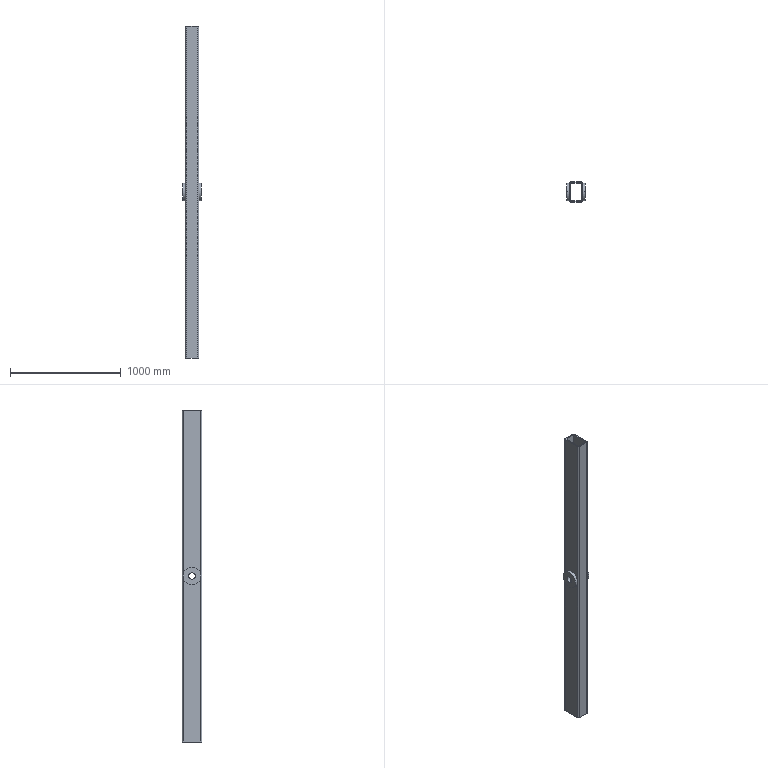Part | SolidWorks | features ICE 2, Extrusion 1, MirrorPattern 1 | 1 solid | 34 faces | box 170 x 180 x 3000 mm | volume 17246858 mm3 | plane 18 | cylinder 16 | commonest cylinder face diameters 4 x4 24 x4 60 x4 160 x4
STEP:
#1=CARTESIAN_POINT('',(-85.,0.,-80.));
#2=VERTEX_POINT('',#1);
#3=CARTESIAN_POINT('',(-85.,0.,80.));
#4=VERTEX_POINT('',#3);
#5=CARTESIAN_POINT('',(-85.,0.,0.));
#6=DIRECTION('',(1.,0.,0.));
#7=DIRECTION('',(0.,0.,-1.));
#8=AXIS2_PLACEMENT_3D('',#5,#6,#7);
#9=CIRCLE('',#8,80.);
#10=EDGE_CURVE('',#2,#4,#9,.T.);
#11=ORIENTED_EDGE('',*,*,#10,.T.);
#12=CARTESIAN_POINT('',(-60.,0.,80.));
#13=VERTEX_POINT('',#12);
#14=CARTESIAN_POINT('',(-85.,0.,80.));
#15=DIRECTION('',(1.,0.,0.));
#16=VECTOR('',#15,1000.);
#17=LINE('',#14,#16);
#18=EDGE_CURVE('',#4,#13,#17,.T.);
#19=ORIENTED_EDGE('',*,*,#18,.T.);
#20=CARTESIAN_POINT('',(-60.,78.,17.776));
#21=VERTEX_POINT('',#20);
#22=CARTESIAN_POINT('',(-60.,0.,0.));
#23=DIRECTION('',(1.,0.,0.));
#24=DIRECTION('',(0.,0.,-1.));
#25=AXIS2_PLACEMENT_3D('',#22,#23,#24);
#26=CIRCLE('',#25,80.);
#27=EDGE_CURVE('',#21,#13,#26,.T.);
#28=ORIENTED_EDGE('',*,*,#27,.F.);
#29=CARTESIAN_POINT('',(-60.,78.,-17.776));
#30=VERTEX_POINT('',#29);
#31=CARTESIAN_POINT('',(-60.,0.,0.));
#32=DIRECTION('',(1.,0.,0.));
#33=DIRECTION('',(0.,0.,-1.));
#34=AXIS2_PLACEMENT_3D('',#31,#32,#33);
#35=CIRCLE('',#34,80.);
#36=EDGE_CURVE('',#30,#21,#35,.T.);
#37=ORIENTED_EDGE('',*,*,#36,.F.);
#38=CARTESIAN_POINT('',(-60.,0.,-80.));
#39=VERTEX_POINT('',#38);
#40=CARTESIAN_POINT('',(-60.,0.,0.));
#41=DIRECTION('',(1.,0.,0.));
#42=DIRECTION('',(0.,0.,-1.));
#43=AXIS2_PLACEMENT_3D('',#40,#41,#42);
#44=CIRCLE('',#43,80.);
#45=EDGE_CURVE('',#39,#30,#44,.T.);
#46=ORIENTED_EDGE('',*,*,#45,.F.);
#47=CARTESIAN_POINT('',(-85.,0.,-80.));
#48=DIRECTION('',(1.,0.,0.));
#49=VECTOR('',#48,1000.);
#50=LINE('',#47,#49);
#51=EDGE_CURVE('',#2,#39,#50,.T.);
#52=ORIENTED_EDGE('',*,*,#51,.F.);
#53=EDGE_LOOP('',(#11,#19,#28,#37,#46,#52));
#54=FACE_OUTER_BOUND('',#53,.T.);
#55=CARTESIAN_POINT('',(-85.,0.,0.));
#56=DIRECTION('',(1.,0.,0.));
#57=DIRECTION('',(0.,0.,-1.));
#58=AXIS2_PLACEMENT_3D('',#55,#56,#57);
#59=CYLINDRICAL_SURFACE('',#58,80.);
#60=ADVANCED_FACE('',(#54),#59,.T.);
#61=CARTESIAN_POINT('',(85.,0.,-80.));
#62=VERTEX_POINT('',#61);
#63=CARTESIAN_POINT('',(85.,0.,80.));
#64=VERTEX_POINT('',#63);
#65=CARTESIAN_POINT('',(85.,0.,0.));
#66=DIRECTION('',(1.,0.,0.));
#67=DIRECTION('',(0.,0.,-1.));
#68=AXIS2_PLACEMENT_3D('',#65,#66,#67);
#69=CIRCLE('',#68,80.);
#70=EDGE_CURVE('',#62,#64,#69,.T.);
#71=ORIENTED_EDGE('',*,*,#70,.F.);
#72=CARTESIAN_POINT('',(60.,0.,-80.));
#73=VERTEX_POINT('',#72);
#74=CARTESIAN_POINT('',(85.,0.,-80.));
#75=DIRECTION('',(-1.,0.,0.));
#76=VECTOR('',#75,1000.);
#77=LINE('',#74,#76);
#78=EDGE_CURVE('',#62,#73,#77,.T.);
#79=ORIENTED_EDGE('',*,*,#78,.T.);
#80=CARTESIAN_POINT('',(60.,78.,-17.776));
#81=VERTEX_POINT('',#80);
#82=CARTESIAN_POINT('',(60.,0.,0.));
#83=DIRECTION('',(1.,0.,0.));
#84=DIRECTION('',(0.,0.,-1.));
#85=AXIS2_PLACEMENT_3D('',#82,#83,#84);
#86=CIRCLE('',#85,80.);
#87=EDGE_CURVE('',#73,#81,#86,.T.);
#88=ORIENTED_EDGE('',*,*,#87,.T.);
#89=CARTESIAN_POINT('',(60.,78.,17.776));
#90=VERTEX_POINT('',#89);
#91=CARTESIAN_POINT('',(60.,0.,0.));
#92=DIRECTION('',(1.,0.,0.));
#93=DIRECTION('',(0.,0.,-1.));
#94=AXIS2_PLACEMENT_3D('',#91,#92,#93);
#95=CIRCLE('',#94,80.);
#96=EDGE_CURVE('',#81,#90,#95,.T.);
#97=ORIENTED_EDGE('',*,*,#96,.T.);
#98=CARTESIAN_POINT('',(60.,0.,80.));
#99=VERTEX_POINT('',#98);
#100=CARTESIAN_POINT('',(60.,0.,0.));
#101=DIRECTION('',(1.,0.,0.));
#102=DIRECTION('',(0.,0.,-1.));
#103=AXIS2_PLACEMENT_3D('',#100,#101,#102);
#104=CIRCLE('',#103,80.);
#105=EDGE_CURVE('',#90,#99,#104,.T.);
#106=ORIENTED_EDGE('',*,*,#105,.T.);
#107=CARTESIAN_POINT('',(85.,0.,80.));
#108=DIRECTION('',(-1.,0.,0.));
#109=VECTOR('',#108,1000.);
#110=LINE('',#107,#109);
#111=EDGE_CURVE('',#64,#99,#110,.T.);
#112=ORIENTED_EDGE('',*,*,#111,.F.);
#113=EDGE_LOOP('',(#71,#79,#88,#97,#106,#112));
#114=FACE_OUTER_BOUND('',#113,.T.);
#115=CARTESIAN_POINT('',(85.,0.,0.));
#116=DIRECTION('',(-1.,0.,0.));
#117=DIRECTION('',(0.,0.,1.));
#118=AXIS2_PLACEMENT_3D('',#115,#116,#117);
#119=CYLINDRICAL_SURFACE('',#118,80.);
#120=ADVANCED_FACE('',(#114),#119,.T.);
#121=CARTESIAN_POINT('',(-85.,0.,30.));
#122=VERTEX_POINT('',#121);
#123=CARTESIAN_POINT('',(-85.,0.,-30.));
#124=VERTEX_POINT('',#123);
#125=CARTESIAN_POINT('',(-85.,0.,0.));
#126=DIRECTION('',(1.,0.,0.));
#127=DIRECTION('',(0.,0.,-1.));
#128=AXIS2_PLACEMENT_3D('',#125,#126,#127);
#129=CIRCLE('',#128,30.);
#130=EDGE_CURVE('',#122,#124,#129,.T.);
#131=ORIENTED_EDGE('',*,*,#130,.F.);
#132=CARTESIAN_POINT('',(-50.,0.,30.));
#133=VERTEX_POINT('',#132);
#134=CARTESIAN_POINT('',(-60.,0.,30.));
#135=DIRECTION('',(1.,0.,0.));
#136=VECTOR('',#135,1000.);
#137=LINE('',#134,#136);
#138=EDGE_CURVE('',#122,#133,#137,.T.);
#139=ORIENTED_EDGE('',*,*,#138,.T.);
#140=CARTESIAN_POINT('',(-50.,0.,-30.));
#141=VERTEX_POINT('',#140);
#142=CARTESIAN_POINT('',(-50.,0.,0.));
#143=DIRECTION('',(1.,0.,0.));
#144=DIRECTION('',(0.,1.,0.));
#145=AXIS2_PLACEMENT_3D('',#142,#143,#144);
#146=CIRCLE('',#145,30.);
#147=EDGE_CURVE('',#133,#141,#146,.T.);
#148=ORIENTED_EDGE('',*,*,#147,.T.);
#149=CARTESIAN_POINT('',(-60.,0.,-30.));
#150=DIRECTION('',(1.,0.,0.));
#151=VECTOR('',#150,1000.);
#152=LINE('',#149,#151);
#153=EDGE_CURVE('',#124,#141,#152,.T.);
#154=ORIENTED_EDGE('',*,*,#153,.F.);
#155=EDGE_LOOP('',(#131,#139,#148,#154));
#156=FACE_OUTER_BOUND('',#155,.T.);
#157=CARTESIAN_POINT('',(-60.,0.,0.));
#158=DIRECTION('',(1.,0.,0.));
#159=DIRECTION('',(0.,0.,-1.));
#160=AXIS2_PLACEMENT_3D('',#157,#158,#159);
#161=CYLINDRICAL_SURFACE('',#160,30.);
#162=ADVANCED_FACE('',(#156),#161,.F.);
#163=CARTESIAN_POINT('',(50.,0.,-30.));
#164=VERTEX_POINT('',#163);
#165=CARTESIAN_POINT('',(50.,0.,30.));
#166=VERTEX_POINT('',#165);
#167=CARTESIAN_POINT('',(50.,0.,0.));
#168=DIRECTION('',(-1.,0.,0.));
#169=DIRECTION('',(0.,0.,1.));
#170=AXIS2_PLACEMENT_3D('',#167,#168,#169);
#171=CIRCLE('',#170,30.);
#172=EDGE_CURVE('',#164,#166,#171,.T.);
#173=ORIENTED_EDGE('',*,*,#172,.T.);
#174=CARTESIAN_POINT('',(85.,0.,30.));
#175=VERTEX_POINT('',#174);
#176=CARTESIAN_POINT('',(-60.,0.,30.));
#177=DIRECTION('',(1.,0.,0.));
#178=VECTOR('',#177,1000.);
#179=LINE('',#176,#178);
#180=EDGE_CURVE('',#166,#175,#179,.T.);
#181=ORIENTED_EDGE('',*,*,#180,.T.);
#182=CARTESIAN_POINT('',(85.,0.,-30.));
#183=VERTEX_POINT('',#182);
#184=CARTESIAN_POINT('',(85.,0.,0.));
#185=DIRECTION('',(1.,0.,0.));
#186=DIRECTION('',(0.,0.,-1.));
#187=AXIS2_PLACEMENT_3D('',#184,#185,#186);
#188=CIRCLE('',#187,30.);
#189=EDGE_CURVE('',#175,#183,#188,.T.);
#190=ORIENTED_EDGE('',*,*,#189,.T.);
#191=CARTESIAN_POINT('',(-60.,0.,-30.));
#192=DIRECTION('',(1.,0.,0.));
#193=VECTOR('',#192,1000.);
#194=LINE('',#191,#193);
#195=EDGE_CURVE('',#164,#183,#194,.T.);
#196=ORIENTED_EDGE('',*,*,#195,.F.);
#197=EDGE_LOOP('',(#173,#181,#190,#196));
#198=FACE_OUTER_BOUND('',#197,.T.);
#199=CARTESIAN_POINT('',(-60.,0.,0.));
#200=DIRECTION('',(1.,0.,0.));
#201=DIRECTION('',(0.,0.,-1.));
#202=AXIS2_PLACEMENT_3D('',#199,#200,#201);
#203=CYLINDRICAL_SURFACE('',#202,30.);
#204=ADVANCED_FACE('',(#198),#203,.F.);
#205=CARTESIAN_POINT('',(-60.,78.,1500.));
#206=VERTEX_POINT('',#205);
#207=CARTESIAN_POINT('',(-60.,78.,1500.));
#208=DIRECTION('',(0.,0.,-1.));
#209=VECTOR('',#208,1000.);
#210=LINE('',#207,#209);
#211=EDGE_CURVE('',#206,#21,#210,.T.);
#212=ORIENTED_EDGE('',*,*,#211,.T.);
#213=ORIENTED_EDGE('',*,*,#27,.T.);
#214=CARTESIAN_POINT('',(-60.,-78.,17.776));
#215=VERTEX_POINT('',#214);
#216=CARTESIAN_POINT('',(-60.,0.,0.));
#217=DIRECTION('',(1.,0.,0.));
#218=DIRECTION('',(0.,0.,-1.));
#219=AXIS2_PLACEMENT_3D('',#216,#217,#218);
#220=CIRCLE('',#219,80.);
#221=EDGE_CURVE('',#13,#215,#220,.T.);
#222=ORIENTED_EDGE('',*,*,#221,.T.);
#223=CARTESIAN_POINT('',(-60.,-78.,1500.));
#224=VERTEX_POINT('',#223);
#225=CARTESIAN_POINT('',(-60.,-78.,1500.));
#226=DIRECTION('',(0.,0.,-1.));
#227=VECTOR('',#226,1000.);
#228=LINE('',#225,#227);
#229=EDGE_CURVE('',#224,#215,#228,.T.);
#230=ORIENTED_EDGE('',*,*,#229,.F.);
#231=CARTESIAN_POINT('',(-60.,78.,1500.));
#232=DIRECTION('',(0.,-1.,0.));
#233=VECTOR('',#232,1000.);
#234=LINE('',#231,#233);
#235=EDGE_CURVE('',#206,#224,#234,.T.);
#236=ORIENTED_EDGE('',*,*,#235,.F.);
#237=EDGE_LOOP('',(#212,#213,#222,#230,#236));
#238=FACE_OUTER_BOUND('',#237,.T.);
#239=CARTESIAN_POINT('',(-60.,-78.,1500.));
#240=DIRECTION('',(1.,0.,0.));
#241=DIRECTION('',(0.,1.,0.));
#242=AXIS2_PLACEMENT_3D('',#239,#240,#241);
#243=PLANE('',#242);
#244=ADVANCED_FACE('',(#238),#243,.F.);
#245=CARTESIAN_POINT('',(60.,-78.,-17.776));
#246=VERTEX_POINT('',#245);
#247=CARTESIAN_POINT('',(60.,0.,0.));
#248=DIRECTION('',(1.,0.,0.));
#249=DIRECTION('',(0.,0.,-1.));
#250=AXIS2_PLACEMENT_3D('',#247,#248,#249);
#251=CIRCLE('',#250,80.);
#252=EDGE_CURVE('',#246,#73,#251,.T.);
#253=ORIENTED_EDGE('',*,*,#252,.F.);
#254=CARTESIAN_POINT('',(60.,-78.,-1500.));
#255=VERTEX_POINT('',#254);
#256=CARTESIAN_POINT('',(60.,-78.,1500.));
#257=DIRECTION('',(0.,0.,-1.));
#258=VECTOR('',#257,1000.);
#259=LINE('',#256,#258);
#260=EDGE_CURVE('',#246,#255,#259,.T.);
#261=ORIENTED_EDGE('',*,*,#260,.T.);
#262=CARTESIAN_POINT('',(60.,78.,-1500.));
#263=VERTEX_POINT('',#262);
#264=CARTESIAN_POINT('',(60.,78.,-1500.));
#265=DIRECTION('',(0.,1.,0.));
#266=VECTOR('',#265,1000.);
#267=LINE('',#264,#266);
#268=EDGE_CURVE('',#255,#263,#267,.T.);
#269=ORIENTED_EDGE('',*,*,#268,.T.);
#270=CARTESIAN_POINT('',(60.,78.,1500.));
#271=DIRECTION('',(0.,0.,-1.));
#272=VECTOR('',#271,1000.);
#273=LINE('',#270,#272);
#274=EDGE_CURVE('',#81,#263,#273,.T.);
#275=ORIENTED_EDGE('',*,*,#274,.F.);
#276=ORIENTED_EDGE('',*,*,#87,.F.);
#277=EDGE_LOOP('',(#253,#261,#269,#275,#276));
#278=FACE_OUTER_BOUND('',#277,.T.);
#279=CARTESIAN_POINT('',(60.,78.,1500.));
#280=DIRECTION('',(-1.,0.,0.));
#281=DIRECTION('',(0.,0.,1.));
#282=AXIS2_PLACEMENT_3D('',#279,#280,#281);
#283=PLANE('',#282);
#284=ADVANCED_FACE('',(#278),#283,.F.);
#285=ORIENTED_EDGE('',*,*,#105,.F.);
#286=CARTESIAN_POINT('',(60.,78.,1500.));
#287=VERTEX_POINT('',#286);
#288=CARTESIAN_POINT('',(60.,78.,1500.));
#289=DIRECTION('',(0.,0.,-1.));
#290=VECTOR('',#289,1000.);
#291=LINE('',#288,#290);
#292=EDGE_CURVE('',#287,#90,#291,.T.);
#293=ORIENTED_EDGE('',*,*,#292,.F.);
#294=CARTESIAN_POINT('',(60.,-78.,1500.));
#295=VERTEX_POINT('',#294);
#296=CARTESIAN_POINT('',(60.,78.,1500.));
#297=DIRECTION('',(0.,1.,0.));
#298=VECTOR('',#297,1000.);
#299=LINE('',#296,#298);
#300=EDGE_CURVE('',#295,#287,#299,.T.);
#301=ORIENTED_EDGE('',*,*,#300,.F.);
#302=CARTESIAN_POINT('',(60.,-78.,17.776));
#303=VERTEX_POINT('',#302);
#304=CARTESIAN_POINT('',(60.,-78.,1500.));
#305=DIRECTION('',(0.,0.,-1.));
#306=VECTOR('',#305,1000.);
#307=LINE('',#304,#306);
#308=EDGE_CURVE('',#295,#303,#307,.T.);
#309=ORIENTED_EDGE('',*,*,#308,.T.);
#310=CARTESIAN_POINT('',(60.,0.,0.));
#311=DIRECTION('',(1.,0.,0.));
#312=DIRECTION('',(0.,0.,-1.));
#313=AXIS2_PLACEMENT_3D('',#310,#311,#312);
#314=CIRCLE('',#313,80.);
#315=EDGE_CURVE('',#99,#303,#314,.T.);
#316=ORIENTED_EDGE('',*,*,#315,.F.);
#317=EDGE_LOOP('',(#285,#293,#301,#309,#316));
#318=FACE_OUTER_BOUND('',#317,.T.);
#319=CARTESIAN_POINT('',(60.,78.,1500.));
#320=DIRECTION('',(-1.,0.,0.));
#321=DIRECTION('',(0.,0.,1.));
#322=AXIS2_PLACEMENT_3D('',#319,#320,#321);
#323=PLANE('',#322);
#324=ADVANCED_FACE('',(#318),#323,.F.);
#325=CARTESIAN_POINT('',(-48.,90.,1500.));
#326=VERTEX_POINT('',#325);
#327=CARTESIAN_POINT('',(-48.,78.,1500.));
#328=DIRECTION('',(0.,0.,1.));
#329=DIRECTION('',(1.,0.,0.));
#330=AXIS2_PLACEMENT_3D('',#327,#328,#329);
#331=CIRCLE('',#330,12.);
#332=EDGE_CURVE('',#326,#206,#331,.T.);
#333=ORIENTED_EDGE('',*,*,#332,.T.);
#334=ORIENTED_EDGE('',*,*,#235,.T.);
#335=CARTESIAN_POINT('',(-48.,-90.,1500.));
#336=VERTEX_POINT('',#335);
#337=CARTESIAN_POINT('',(-48.,-78.,1500.));
#338=DIRECTION('',(0.,0.,1.));
#339=DIRECTION('',(-1.,0.,0.));
#340=AXIS2_PLACEMENT_3D('',#337,#338,#339);
#341=CIRCLE('',#340,12.);
#342=EDGE_CURVE('',#224,#336,#341,.T.);
#343=ORIENTED_EDGE('',*,*,#342,.T.);
#344=CARTESIAN_POINT('',(48.,-90.,1500.));
#345=VERTEX_POINT('',#344);
#346=CARTESIAN_POINT('',(0.,-90.,1500.));
#347=DIRECTION('',(1.,0.,0.));
#348=VECTOR('',#347,1000.);
#349=LINE('',#346,#348);
#350=EDGE_CURVE('',#336,#345,#349,.T.);
#351=ORIENTED_EDGE('',*,*,#350,.T.);
#352=CARTESIAN_POINT('',(48.,-78.,1500.));
#353=DIRECTION('',(0.,0.,1.));
#354=DIRECTION('',(1.,0.,0.));
#355=AXIS2_PLACEMENT_3D('',#352,#353,#354);
#356=CIRCLE('',#355,12.);
#357=EDGE_CURVE('',#345,#295,#356,.T.);
#358=ORIENTED_EDGE('',*,*,#357,.T.);
#359=ORIENTED_EDGE('',*,*,#300,.T.);
#360=CARTESIAN_POINT('',(48.,90.,1500.));
#361=VERTEX_POINT('',#360);
#362=CARTESIAN_POINT('',(48.,78.,1500.));
#363=DIRECTION('',(0.,0.,1.));
#364=DIRECTION('',(-1.,0.,0.));
#365=AXIS2_PLACEMENT_3D('',#362,#363,#364);
#366=CIRCLE('',#365,12.);
#367=EDGE_CURVE('',#287,#361,#366,.T.);
#368=ORIENTED_EDGE('',*,*,#367,.T.);
#369=CARTESIAN_POINT('',(0.,90.,1500.));
#370=DIRECTION('',(-1.,0.,0.));
#371=VECTOR('',#370,1000.);
#372=LINE('',#369,#371);
#373=EDGE_CURVE('',#361,#326,#372,.T.);
#374=ORIENTED_EDGE('',*,*,#373,.T.);
#375=EDGE_LOOP('',(#333,#334,#343,#351,#358,#359,#368,#374));
#376=FACE_OUTER_BOUND('',#375,.T.);
#377=CARTESIAN_POINT('',(-50.,78.,1500.));
#378=VERTEX_POINT('',#377);
#379=CARTESIAN_POINT('',(-50.,-78.,1500.));
#380=VERTEX_POINT('',#379);
#381=CARTESIAN_POINT('',(-50.,78.,1500.));
#382=DIRECTION('',(0.,-1.,0.));
#383=VECTOR('',#382,1000.);
#384=LINE('',#381,#383);
#385=EDGE_CURVE('',#378,#380,#384,.T.);
#386=ORIENTED_EDGE('',*,*,#385,.F.);
#387=CARTESIAN_POINT('',(-48.,80.,1500.));
#388=VERTEX_POINT('',#387);
#389=CARTESIAN_POINT('',(-48.,78.,1500.));
#390=DIRECTION('',(0.,0.,1.));
#391=DIRECTION('',(1.,0.,0.));
#392=AXIS2_PLACEMENT_3D('',#389,#390,#391);
#393=CIRCLE('',#392,2.);
#394=EDGE_CURVE('',#388,#378,#393,.T.);
#395=ORIENTED_EDGE('',*,*,#394,.F.);
#396=CARTESIAN_POINT('',(48.,80.,1500.));
#397=VERTEX_POINT('',#396);
#398=CARTESIAN_POINT('',(0.,80.,1500.));
#399=DIRECTION('',(-1.,0.,0.));
#400=VECTOR('',#399,1000.);
#401=LINE('',#398,#400);
#402=EDGE_CURVE('',#397,#388,#401,.T.);
#403=ORIENTED_EDGE('',*,*,#402,.F.);
#404=CARTESIAN_POINT('',(50.,78.,1500.));
#405=VERTEX_POINT('',#404);
#406=CARTESIAN_POINT('',(48.,78.,1500.));
#407=DIRECTION('',(0.,0.,1.));
#408=DIRECTION('',(-1.,0.,0.));
#409=AXIS2_PLACEMENT_3D('',#406,#407,#408);
#410=CIRCLE('',#409,2.);
#411=EDGE_CURVE('',#405,#397,#410,.T.);
#412=ORIENTED_EDGE('',*,*,#411,.F.);
#413=CARTESIAN_POINT('',(50.,-78.,1500.));
#414=VERTEX_POINT('',#413);
#415=CARTESIAN_POINT('',(50.,78.,1500.));
#416=DIRECTION('',(0.,1.,0.));
#417=VECTOR('',#416,1000.);
#418=LINE('',#415,#417);
#419=EDGE_CURVE('',#414,#405,#418,.T.);
#420=ORIENTED_EDGE('',*,*,#419,.F.);
#421=CARTESIAN_POINT('',(48.,-80.,1500.));
#422=VERTEX_POINT('',#421);
#423=CARTESIAN_POINT('',(48.,-78.,1500.));
#424=DIRECTION('',(0.,0.,1.));
#425=DIRECTION('',(1.,0.,0.));
#426=AXIS2_PLACEMENT_3D('',#423,#424,#425);
#427=CIRCLE('',#426,2.);
#428=EDGE_CURVE('',#422,#414,#427,.T.);
#429=ORIENTED_EDGE('',*,*,#428,.F.);
#430=CARTESIAN_POINT('',(-48.,-80.,1500.));
#431=VERTEX_POINT('',#430);
#432=CARTESIAN_POINT('',(0.,-80.,1500.));
#433=DIRECTION('',(1.,0.,0.));
#434=VECTOR('',#433,1000.);
#435=LINE('',#432,#434);
#436=EDGE_CURVE('',#431,#422,#435,.T.);
#437=ORIENTED_EDGE('',*,*,#436,.F.);
#438=CARTESIAN_POINT('',(-48.,-78.,1500.));
#439=DIRECTION('',(0.,0.,1.));
#440=DIRECTION('',(-1.,0.,0.));
#441=AXIS2_PLACEMENT_3D('',#438,#439,#440);
#442=CIRCLE('',#441,2.);
#443=EDGE_CURVE('',#380,#431,#442,.T.);
#444=ORIENTED_EDGE('',*,*,#443,.F.);
#445=EDGE_LOOP('',(#386,#395,#403,#412,#420,#429,#437,#444));
#446=FACE_BOUND('',#445,.T.);
#447=CARTESIAN_POINT('',(-48.,78.,1500.));
#448=DIRECTION('',(0.,0.,1.));
#449=DIRECTION('',(1.,0.,0.));
#450=AXIS2_PLACEMENT_3D('',#447,#448,#449);
#451=PLANE('',#450);
#452=ADVANCED_FACE('',(#376,#446),#451,.T.);
#453=CARTESIAN_POINT('',(-48.,90.,-1500.));
#454=VERTEX_POINT('',#453);
#455=CARTESIAN_POINT('',(-60.,78.,-1500.));
#456=VERTEX_POINT('',#455);
#457=CARTESIAN_POINT('',(-48.,78.,-1500.));
#458=DIRECTION('',(0.,0.,1.));
#459=DIRECTION('',(1.,0.,0.));
#460=AXIS2_PLACEMENT_3D('',#457,#458,#459);
#461=CIRCLE('',#460,12.);
#462=EDGE_CURVE('',#454,#456,#461,.T.);
#463=ORIENTED_EDGE('',*,*,#462,.F.);
#464=CARTESIAN_POINT('',(48.,90.,-1500.));
#465=VERTEX_POINT('',#464);
#466=CARTESIAN_POINT('',(0.,90.,-1500.));
#467=DIRECTION('',(-1.,0.,0.));
#468=VECTOR('',#467,1000.);
#469=LINE('',#466,#468);
#470=EDGE_CURVE('',#465,#454,#469,.T.);
#471=ORIENTED_EDGE('',*,*,#470,.F.);
#472=CARTESIAN_POINT('',(48.,78.,-1500.));
#473=DIRECTION('',(0.,0.,1.));
#474=DIRECTION('',(-1.,0.,0.));
#475=AXIS2_PLACEMENT_3D('',#472,#473,#474);
#476=CIRCLE('',#475,12.);
#477=EDGE_CURVE('',#263,#465,#476,.T.);
#478=ORIENTED_EDGE('',*,*,#477,.F.);
#479=ORIENTED_EDGE('',*,*,#268,.F.);
#480=CARTESIAN_POINT('',(48.,-90.,-1500.));
#481=VERTEX_POINT('',#480);
#482=CARTESIAN_POINT('',(48.,-78.,-1500.));
#483=DIRECTION('',(0.,0.,1.));
#484=DIRECTION('',(1.,0.,0.));
#485=AXIS2_PLACEMENT_3D('',#482,#483,#484);
#486=CIRCLE('',#485,12.);
#487=EDGE_CURVE('',#481,#255,#486,.T.);
#488=ORIENTED_EDGE('',*,*,#487,.F.);
#489=CARTESIAN_POINT('',(-48.,-90.,-1500.));
#490=VERTEX_POINT('',#489);
#491=CARTESIAN_POINT('',(0.,-90.,-1500.));
#492=DIRECTION('',(1.,0.,0.));
#493=VECTOR('',#492,1000.);
#494=LINE('',#491,#493);
#495=EDGE_CURVE('',#490,#481,#494,.T.);
#496=ORIENTED_EDGE('',*,*,#495,.F.);
#497=CARTESIAN_POINT('',(-60.,-78.,-1500.));
#498=VERTEX_POINT('',#497);
#499=CARTESIAN_POINT('',(-48.,-78.,-1500.));
#500=DIRECTION('',(0.,0.,1.));
#501=DIRECTION('',(-1.,0.,0.));
#502=AXIS2_PLACEMENT_3D('',#499,#500,#501);
#503=CIRCLE('',#502,12.);
#504=EDGE_CURVE('',#498,#490,#503,.T.);
#505=ORIENTED_EDGE('',*,*,#504,.F.);
#506=CARTESIAN_POINT('',(-60.,-78.,-1500.));
#507=DIRECTION('',(0.,-1.,0.));
#508=VECTOR('',#507,1000.);
#509=LINE('',#506,#508);
#510=EDGE_CURVE('',#456,#498,#509,.T.);
#511=ORIENTED_EDGE('',*,*,#510,.F.);
#512=EDGE_LOOP('',(#463,#471,#478,#479,#488,#496,#505,#511));
#513=FACE_OUTER_BOUND('',#512,.T.);
#514=CARTESIAN_POINT('',(-48.,80.,-1500.));
#515=VERTEX_POINT('',#514);
#516=CARTESIAN_POINT('',(-50.,78.,-1500.));
#517=VERTEX_POINT('',#516);
#518=CARTESIAN_POINT('',(-48.,78.,-1500.));
#519=DIRECTION('',(0.,0.,1.));
#520=DIRECTION('',(1.,0.,0.));
#521=AXIS2_PLACEMENT_3D('',#518,#519,#520);
#522=CIRCLE('',#521,2.);
#523=EDGE_CURVE('',#515,#517,#522,.T.);
#524=ORIENTED_EDGE('',*,*,#523,.T.);
#525=CARTESIAN_POINT('',(-50.,-78.,-1500.));
#526=VERTEX_POINT('',#525);
#527=CARTESIAN_POINT('',(-50.,-78.,-1500.));
#528=DIRECTION('',(0.,-1.,0.));
#529=VECTOR('',#528,1000.);
#530=LINE('',#527,#529);
#531=EDGE_CURVE('',#517,#526,#530,.T.);
#532=ORIENTED_EDGE('',*,*,#531,.T.);
#533=CARTESIAN_POINT('',(-48.,-80.,-1500.));
#534=VERTEX_POINT('',#533);
#535=CARTESIAN_POINT('',(-48.,-78.,-1500.));
#536=DIRECTION('',(0.,0.,1.));
#537=DIRECTION('',(-1.,0.,0.));
#538=AXIS2_PLACEMENT_3D('',#535,#536,#537);
#539=CIRCLE('',#538,2.);
#540=EDGE_CURVE('',#526,#534,#539,.T.);
#541=ORIENTED_EDGE('',*,*,#540,.T.);
#542=CARTESIAN_POINT('',(48.,-80.,-1500.));
#543=VERTEX_POINT('',#542);
#544=CARTESIAN_POINT('',(0.,-80.,-1500.));
#545=DIRECTION('',(1.,0.,0.));
#546=VECTOR('',#545,1000.);
#547=LINE('',#544,#546);
#548=EDGE_CURVE('',#534,#543,#547,.T.);
#549=ORIENTED_EDGE('',*,*,#548,.T.);
#550=CARTESIAN_POINT('',(50.,-78.,-1500.));
#551=VERTEX_POINT('',#550);
#552=CARTESIAN_POINT('',(48.,-78.,-1500.));
#553=DIRECTION('',(0.,0.,1.));
#554=DIRECTION('',(1.,0.,0.));
#555=AXIS2_PLACEMENT_3D('',#552,#553,#554);
#556=CIRCLE('',#555,2.);
#557=EDGE_CURVE('',#543,#551,#556,.T.);
#558=ORIENTED_EDGE('',*,*,#557,.T.);
#559=CARTESIAN_POINT('',(50.,78.,-1500.));
#560=VERTEX_POINT('',#559);
#561=CARTESIAN_POINT('',(50.,78.,-1500.));
#562=DIRECTION('',(0.,1.,0.));
#563=VECTOR('',#562,1000.);
#564=LINE('',#561,#563);
#565=EDGE_CURVE('',#551,#560,#564,.T.);
#566=ORIENTED_EDGE('',*,*,#565,.T.);
#567=CARTESIAN_POINT('',(48.,80.,-1500.));
#568=VERTEX_POINT('',#567);
#569=CARTESIAN_POINT('',(48.,78.,-1500.));
#570=DIRECTION('',(0.,0.,1.));
#571=DIRECTION('',(-1.,0.,0.));
#572=AXIS2_PLACEMENT_3D('',#569,#570,#571);
#573=CIRCLE('',#572,2.);
#574=EDGE_CURVE('',#560,#568,#573,.T.);
#575=ORIENTED_EDGE('',*,*,#574,.T.);
#576=CARTESIAN_POINT('',(0.,80.,-1500.));
#577=DIRECTION('',(-1.,0.,0.));
#578=VECTOR('',#577,1000.);
#579=LINE('',#576,#578);
#580=EDGE_CURVE('',#568,#515,#579,.T.);
#581=ORIENTED_EDGE('',*,*,#580,.T.);
#582=EDGE_LOOP('',(#524,#532,#541,#549,#558,#566,#575,#581));
#583=FACE_BOUND('',#582,.T.);
#584=CARTESIAN_POINT('',(-48.,78.,-1500.));
#585=DIRECTION('',(0.,0.,1.));
#586=DIRECTION('',(1.,0.,0.));
#587=AXIS2_PLACEMENT_3D('',#584,#585,#586);
#588=PLANE('',#587);
#589=ADVANCED_FACE('',(#513,#583),#588,.F.);
#590=ORIENTED_EDGE('',*,*,#462,.T.);
#591=CARTESIAN_POINT('',(-60.,78.,1500.));
#592=DIRECTION('',(0.,0.,-1.));
#593=VECTOR('',#592,1000.);
#594=LINE('',#591,#593);
#595=EDGE_CURVE('',#30,#456,#594,.T.);
#596=ORIENTED_EDGE('',*,*,#595,.F.);
#597=CARTESIAN_POINT('',(-60.,78.,1500.));
#598=DIRECTION('',(0.,0.,-1.));
#599=VECTOR('',#598,1000.);
#600=LINE('',#597,#599);
#601=EDGE_CURVE('',#21,#30,#600,.T.);
#602=ORIENTED_EDGE('',*,*,#601,.F.);
#603=ORIENTED_EDGE('',*,*,#211,.F.);
#604=ORIENTED_EDGE('',*,*,#332,.F.);
#605=CARTESIAN_POINT('',(-48.,90.,1500.));
#606=DIRECTION('',(0.,0.,-1.));
#607=VECTOR('',#606,1000.);
#608=LINE('',#605,#607);
#609=EDGE_CURVE('',#326,#454,#608,.T.);
#610=ORIENTED_EDGE('',*,*,#609,.T.);
#611=EDGE_LOOP('',(#590,#596,#602,#603,#604,#610));
#612=FACE_OUTER_BOUND('',#611,.T.);
#613=CARTESIAN_POINT('',(-48.,78.,1500.));
#614=DIRECTION('',(0.,0.,-1.));
#615=DIRECTION('',(-1.,0.,0.));
#616=AXIS2_PLACEMENT_3D('',#613,#614,#615);
#617=CYLINDRICAL_SURFACE('',#616,12.);
#618=ADVANCED_FACE('',(#612),#617,.T.);
#619=CARTESIAN_POINT('',(-60.,-78.,-17.776));
#620=VERTEX_POINT('',#619);
#621=CARTESIAN_POINT('',(-60.,-78.,1500.));
#622=DIRECTION('',(0.,0.,-1.));
#623=VECTOR('',#622,1000.);
#624=LINE('',#621,#623);
#625=EDGE_CURVE('',#620,#498,#624,.T.);
#626=ORIENTED_EDGE('',*,*,#625,.F.);
#627=CARTESIAN_POINT('',(-60.,0.,0.));
#628=DIRECTION('',(1.,0.,0.));
#629=DIRECTION('',(0.,0.,-1.));
#630=AXIS2_PLACEMENT_3D('',#627,#628,#629);
#631=CIRCLE('',#630,80.);
#632=EDGE_CURVE('',#620,#39,#631,.T.);
#633=ORIENTED_EDGE('',*,*,#632,.T.);
#634=ORIENTED_EDGE('',*,*,#45,.T.);
#635=ORIENTED_EDGE('',*,*,#595,.T.);
#636=ORIENTED_EDGE('',*,*,#510,.T.);
#637=EDGE_LOOP('',(#626,#633,#634,#635,#636));
#638=FACE_OUTER_BOUND('',#637,.T.);
#639=CARTESIAN_POINT('',(-60.,-78.,1500.));
#640=DIRECTION('',(1.,0.,0.));
#641=DIRECTION('',(0.,1.,0.));
#642=AXIS2_PLACEMENT_3D('',#639,#640,#641);
#643=PLANE('',#642);
#644=ADVANCED_FACE('',(#638),#643,.F.);
#645=ORIENTED_EDGE('',*,*,#504,.T.);
#646=CARTESIAN_POINT('',(-48.,-90.,1500.));
#647=DIRECTION('',(0.,0.,-1.));
#648=VECTOR('',#647,1000.);
#649=LINE('',#646,#648);
#650=EDGE_CURVE('',#336,#490,#649,.T.);
#651=ORIENTED_EDGE('',*,*,#650,.F.);
#652=ORIENTED_EDGE('',*,*,#342,.F.);
#653=ORIENTED_EDGE('',*,*,#229,.T.);
#654=CARTESIAN_POINT('',(-60.,-78.,1500.));
#655=DIRECTION('',(0.,0.,-1.));
#656=VECTOR('',#655,1000.);
#657=LINE('',#654,#656);
#658=EDGE_CURVE('',#215,#620,#657,.T.);
#659=ORIENTED_EDGE('',*,*,#658,.T.);
#660=ORIENTED_EDGE('',*,*,#625,.T.);
#661=EDGE_LOOP('',(#645,#651,#652,#653,#659,#660));
#662=FACE_OUTER_BOUND('',#661,.T.);
#663=CARTESIAN_POINT('',(-48.,-78.,1500.));
#664=DIRECTION('',(0.,0.,-1.));
#665=DIRECTION('',(-1.,0.,0.));
#666=AXIS2_PLACEMENT_3D('',#663,#664,#665);
#667=CYLINDRICAL_SURFACE('',#666,12.);
#668=ADVANCED_FACE('',(#662),#667,.T.);
#669=ORIENTED_EDGE('',*,*,#495,.T.);
#670=CARTESIAN_POINT('',(48.,-90.,1500.));
#671=DIRECTION('',(0.,0.,-1.));
#672=VECTOR('',#671,1000.);
#673=LINE('',#670,#672);
#674=EDGE_CURVE('',#345,#481,#673,.T.);
#675=ORIENTED_EDGE('',*,*,#674,.F.);
#676=ORIENTED_EDGE('',*,*,#350,.F.);
#677=ORIENTED_EDGE('',*,*,#650,.T.);
#678=EDGE_LOOP('',(#669,#675,#676,#677));
#679=FACE_OUTER_BOUND('',#678,.T.);
#680=CARTESIAN_POINT('',(0.,-90.,1500.));
#681=DIRECTION('',(0.,1.,0.));
#682=DIRECTION('',(-1.,0.,0.));
#683=AXIS2_PLACEMENT_3D('',#680,#681,#682);
#684=PLANE('',#683);
#685=ADVANCED_FACE('',(#679),#684,.F.);
#686=ORIENTED_EDGE('',*,*,#487,.T.);
#687=ORIENTED_EDGE('',*,*,#260,.F.);
#688=CARTESIAN_POINT('',(60.,-78.,1500.));
#689=DIRECTION('',(0.,0.,-1.));
#690=VECTOR('',#689,1000.);
#691=LINE('',#688,#690);
#692=EDGE_CURVE('',#303,#246,#691,.T.);
#693=ORIENTED_EDGE('',*,*,#692,.F.);
#694=ORIENTED_EDGE('',*,*,#308,.F.);
#695=ORIENTED_EDGE('',*,*,#357,.F.);
#696=ORIENTED_EDGE('',*,*,#674,.T.);
#697=EDGE_LOOP('',(#686,#687,#693,#694,#695,#696));
#698=FACE_OUTER_BOUND('',#697,.T.);
#699=CARTESIAN_POINT('',(48.,-78.,1500.));
#700=DIRECTION('',(0.,0.,-1.));
#701=DIRECTION('',(-1.,0.,0.));
#702=AXIS2_PLACEMENT_3D('',#699,#700,#701);
#703=CYLINDRICAL_SURFACE('',#702,12.);
#704=ADVANCED_FACE('',(#698),#703,.T.);
#705=ORIENTED_EDGE('',*,*,#477,.T.);
#706=CARTESIAN_POINT('',(48.,90.,1500.));
#707=DIRECTION('',(0.,0.,-1.));
#708=VECTOR('',#707,1000.);
#709=LINE('',#706,#708);
#710=EDGE_CURVE('',#361,#465,#709,.T.);
#711=ORIENTED_EDGE('',*,*,#710,.F.);
#712=ORIENTED_EDGE('',*,*,#367,.F.);
#713=ORIENTED_EDGE('',*,*,#292,.T.);
#714=CARTESIAN_POINT('',(60.,78.,1500.));
#715=DIRECTION('',(0.,0.,-1.));
#716=VECTOR('',#715,1000.);
#717=LINE('',#714,#716);
#718=EDGE_CURVE('',#90,#81,#717,.T.);
#719=ORIENTED_EDGE('',*,*,#718,.T.);
#720=ORIENTED_EDGE('',*,*,#274,.T.);
#721=EDGE_LOOP('',(#705,#711,#712,#713,#719,#720));
#722=FACE_OUTER_BOUND('',#721,.T.);
#723=CARTESIAN_POINT('',(48.,78.,1500.));
#724=DIRECTION('',(0.,0.,-1.));
#725=DIRECTION('',(-1.,0.,0.));
#726=AXIS2_PLACEMENT_3D('',#723,#724,#725);
#727=CYLINDRICAL_SURFACE('',#726,12.);
#728=ADVANCED_FACE('',(#722),#727,.T.);
#729=ORIENTED_EDGE('',*,*,#470,.T.);
#730=ORIENTED_EDGE('',*,*,#609,.F.);
#731=ORIENTED_EDGE('',*,*,#373,.F.);
#732=ORIENTED_EDGE('',*,*,#710,.T.);
#733=EDGE_LOOP('',(#729,#730,#731,#732));
#734=FACE_OUTER_BOUND('',#733,.T.);
#735=CARTESIAN_POINT('',(0.,90.,1500.));
#736=DIRECTION('',(0.,-1.,0.));
#737=DIRECTION('',(0.,0.,-1.));
#738=AXIS2_PLACEMENT_3D('',#735,#736,#737);
#739=PLANE('',#738);
#740=ADVANCED_FACE('',(#734),#739,.F.);
#741=ORIENTED_EDGE('',*,*,#523,.F.);
#742=CARTESIAN_POINT('',(-48.,80.,1500.));
#743=DIRECTION('',(0.,0.,-1.));
#744=VECTOR('',#743,1000.);
#745=LINE('',#742,#744);
#746=EDGE_CURVE('',#388,#515,#745,.T.);
#747=ORIENTED_EDGE('',*,*,#746,.F.);
#748=ORIENTED_EDGE('',*,*,#394,.T.);
#749=CARTESIAN_POINT('',(-50.,78.,1500.));
#750=DIRECTION('',(0.,0.,-1.));
#751=VECTOR('',#750,1000.);
#752=LINE('',#749,#751);
#753=EDGE_CURVE('',#378,#517,#752,.T.);
#754=ORIENTED_EDGE('',*,*,#753,.T.);
#755=EDGE_LOOP('',(#741,#747,#748,#754));
#756=FACE_OUTER_BOUND('',#755,.T.);
#757=CARTESIAN_POINT('',(-48.,78.,1500.));
#758=DIRECTION('',(0.,0.,-1.));
#759=DIRECTION('',(-1.,0.,0.));
#760=AXIS2_PLACEMENT_3D('',#757,#758,#759);
#761=CYLINDRICAL_SURFACE('',#760,2.);
#762=ADVANCED_FACE('',(#756),#761,.F.);
#763=CARTESIAN_POINT('',(-50.,0.,0.));
#764=DIRECTION('',(1.,0.,0.));
#765=DIRECTION('',(0.,1.,0.));
#766=AXIS2_PLACEMENT_3D('',#763,#764,#765);
#767=CIRCLE('',#766,30.);
#768=EDGE_CURVE('',#141,#133,#767,.T.);
#769=ORIENTED_EDGE('',*,*,#768,.F.);
#770=ORIENTED_EDGE('',*,*,#147,.F.);
#771=EDGE_LOOP('',(#769,#770));
#772=FACE_BOUND('',#771,.T.);
#773=ORIENTED_EDGE('',*,*,#531,.F.);
#774=ORIENTED_EDGE('',*,*,#753,.F.);
#775=ORIENTED_EDGE('',*,*,#385,.T.);
#776=CARTESIAN_POINT('',(-50.,-78.,1500.));
#777=DIRECTION('',(0.,0.,-1.));
#778=VECTOR('',#777,1000.);
#779=LINE('',#776,#778);
#780=EDGE_CURVE('',#380,#526,#779,.T.);
#781=ORIENTED_EDGE('',*,*,#780,.T.);
#782=EDGE_LOOP('',(#773,#774,#775,#781));
#783=FACE_OUTER_BOUND('',#782,.T.);
#784=CARTESIAN_POINT('',(-50.,-78.,1500.));
#785=DIRECTION('',(1.,0.,0.));
#786=DIRECTION('',(0.,1.,0.));
#787=AXIS2_PLACEMENT_3D('',#784,#785,#786);
#788=PLANE('',#787);
#789=ADVANCED_FACE('',(#772,#783),#788,.T.);
#790=ORIENTED_EDGE('',*,*,#540,.F.);
#791=ORIENTED_EDGE('',*,*,#780,.F.);
#792=ORIENTED_EDGE('',*,*,#443,.T.);
#793=CARTESIAN_POINT('',(-48.,-80.,1500.));
#794=DIRECTION('',(0.,0.,-1.));
#795=VECTOR('',#794,1000.);
#796=LINE('',#793,#795);
#797=EDGE_CURVE('',#431,#534,#796,.T.);
#798=ORIENTED_EDGE('',*,*,#797,.T.);
#799=EDGE_LOOP('',(#790,#791,#792,#798));
#800=FACE_OUTER_BOUND('',#799,.T.);
#801=CARTESIAN_POINT('',(-48.,-78.,1500.));
#802=DIRECTION('',(0.,0.,-1.));
#803=DIRECTION('',(-1.,0.,0.));
#804=AXIS2_PLACEMENT_3D('',#801,#802,#803);
#805=CYLINDRICAL_SURFACE('',#804,2.);
#806=ADVANCED_FACE('',(#800),#805,.F.);
#807=ORIENTED_EDGE('',*,*,#548,.F.);
#808=ORIENTED_EDGE('',*,*,#797,.F.);
#809=ORIENTED_EDGE('',*,*,#436,.T.);
#810=CARTESIAN_POINT('',(48.,-80.,1500.));
#811=DIRECTION('',(0.,0.,-1.));
#812=VECTOR('',#811,1000.);
#813=LINE('',#810,#812);
#814=EDGE_CURVE('',#422,#543,#813,.T.);
#815=ORIENTED_EDGE('',*,*,#814,.T.);
#816=EDGE_LOOP('',(#807,#808,#809,#815));
#817=FACE_OUTER_BOUND('',#816,.T.);
#818=CARTESIAN_POINT('',(0.,-80.,1500.));
#819=DIRECTION('',(0.,1.,0.));
#820=DIRECTION('',(-1.,0.,0.));
#821=AXIS2_PLACEMENT_3D('',#818,#819,#820);
#822=PLANE('',#821);
#823=ADVANCED_FACE('',(#817),#822,.T.);
#824=ORIENTED_EDGE('',*,*,#557,.F.);
#825=ORIENTED_EDGE('',*,*,#814,.F.);
#826=ORIENTED_EDGE('',*,*,#428,.T.);
#827=CARTESIAN_POINT('',(50.,-78.,1500.));
#828=DIRECTION('',(0.,0.,-1.));
#829=VECTOR('',#828,1000.);
#830=LINE('',#827,#829);
#831=EDGE_CURVE('',#414,#551,#830,.T.);
#832=ORIENTED_EDGE('',*,*,#831,.T.);
#833=EDGE_LOOP('',(#824,#825,#826,#832));
#834=FACE_OUTER_BOUND('',#833,.T.);
#835=CARTESIAN_POINT('',(48.,-78.,1500.));
#836=DIRECTION('',(0.,0.,-1.));
#837=DIRECTION('',(-1.,0.,0.));
#838=AXIS2_PLACEMENT_3D('',#835,#836,#837);
#839=CYLINDRICAL_SURFACE('',#838,2.);
#840=ADVANCED_FACE('',(#834),#839,.F.);
#841=ORIENTED_EDGE('',*,*,#172,.F.);
#842=CARTESIAN_POINT('',(50.,0.,0.));
#843=DIRECTION('',(-1.,0.,0.));
#844=DIRECTION('',(0.,0.,1.));
#845=AXIS2_PLACEMENT_3D('',#842,#843,#844);
#846=CIRCLE('',#845,30.);
#847=EDGE_CURVE('',#166,#164,#846,.T.);
#848=ORIENTED_EDGE('',*,*,#847,.F.);
#849=EDGE_LOOP('',(#841,#848));
#850=FACE_BOUND('',#849,.T.);
#851=ORIENTED_EDGE('',*,*,#565,.F.);
#852=ORIENTED_EDGE('',*,*,#831,.F.);
#853=ORIENTED_EDGE('',*,*,#419,.T.);
#854=CARTESIAN_POINT('',(50.,78.,1500.));
#855=DIRECTION('',(0.,0.,-1.));
#856=VECTOR('',#855,1000.);
#857=LINE('',#854,#856);
#858=EDGE_CURVE('',#405,#560,#857,.T.);
#859=ORIENTED_EDGE('',*,*,#858,.T.);
#860=EDGE_LOOP('',(#851,#852,#853,#859));
#861=FACE_OUTER_BOUND('',#860,.T.);
#862=CARTESIAN_POINT('',(50.,78.,1500.));
#863=DIRECTION('',(-1.,0.,0.));
#864=DIRECTION('',(0.,0.,1.));
#865=AXIS2_PLACEMENT_3D('',#862,#863,#864);
#866=PLANE('',#865);
#867=ADVANCED_FACE('',(#850,#861),#866,.T.);
#868=ORIENTED_EDGE('',*,*,#574,.F.);
#869=ORIENTED_EDGE('',*,*,#858,.F.);
#870=ORIENTED_EDGE('',*,*,#411,.T.);
#871=CARTESIAN_POINT('',(48.,80.,1500.));
#872=DIRECTION('',(0.,0.,-1.));
#873=VECTOR('',#872,1000.);
#874=LINE('',#871,#873);
#875=EDGE_CURVE('',#397,#568,#874,.T.);
#876=ORIENTED_EDGE('',*,*,#875,.T.);
#877=EDGE_LOOP('',(#868,#869,#870,#876));
#878=FACE_OUTER_BOUND('',#877,.T.);
#879=CARTESIAN_POINT('',(48.,78.,1500.));
#880=DIRECTION('',(0.,0.,-1.));
#881=DIRECTION('',(-1.,0.,0.));
#882=AXIS2_PLACEMENT_3D('',#879,#880,#881);
#883=CYLINDRICAL_SURFACE('',#882,2.);
#884=ADVANCED_FACE('',(#878),#883,.F.);
#885=ORIENTED_EDGE('',*,*,#580,.F.);
#886=ORIENTED_EDGE('',*,*,#875,.F.);
#887=ORIENTED_EDGE('',*,*,#402,.T.);
#888=ORIENTED_EDGE('',*,*,#746,.T.);
#889=EDGE_LOOP('',(#885,#886,#887,#888));
#890=FACE_OUTER_BOUND('',#889,.T.);
#891=CARTESIAN_POINT('',(0.,80.,1500.));
#892=DIRECTION('',(0.,-1.,0.));
#893=DIRECTION('',(0.,0.,-1.));
#894=AXIS2_PLACEMENT_3D('',#891,#892,#893);
#895=PLANE('',#894);
#896=ADVANCED_FACE('',(#890),#895,.T.);
#897=ORIENTED_EDGE('',*,*,#180,.F.);
#898=ORIENTED_EDGE('',*,*,#847,.T.);
#899=ORIENTED_EDGE('',*,*,#195,.T.);
#900=CARTESIAN_POINT('',(85.,0.,0.));
#901=DIRECTION('',(1.,0.,0.));
#902=DIRECTION('',(0.,0.,-1.));
#903=AXIS2_PLACEMENT_3D('',#900,#901,#902);
#904=CIRCLE('',#903,30.);
#905=EDGE_CURVE('',#183,#175,#904,.T.);
#906=ORIENTED_EDGE('',*,*,#905,.T.);
#907=EDGE_LOOP('',(#897,#898,#899,#906));
#908=FACE_OUTER_BOUND('',#907,.T.);
#909=CARTESIAN_POINT('',(-60.,0.,0.));
#910=DIRECTION('',(1.,0.,0.));
#911=DIRECTION('',(0.,0.,-1.));
#912=AXIS2_PLACEMENT_3D('',#909,#910,#911);
#913=CYLINDRICAL_SURFACE('',#912,30.);
#914=ADVANCED_FACE('',(#908),#913,.F.);
#915=ORIENTED_EDGE('',*,*,#138,.F.);
#916=CARTESIAN_POINT('',(-85.,0.,0.));
#917=DIRECTION('',(1.,0.,0.));
#918=DIRECTION('',(0.,0.,-1.));
#919=AXIS2_PLACEMENT_3D('',#916,#917,#918);
#920=CIRCLE('',#919,30.);
#921=EDGE_CURVE('',#124,#122,#920,.T.);
#922=ORIENTED_EDGE('',*,*,#921,.F.);
#923=ORIENTED_EDGE('',*,*,#153,.T.);
#924=ORIENTED_EDGE('',*,*,#768,.T.);
#925=EDGE_LOOP('',(#915,#922,#923,#924));
#926=FACE_OUTER_BOUND('',#925,.T.);
#927=CARTESIAN_POINT('',(-60.,0.,0.));
#928=DIRECTION('',(1.,0.,0.));
#929=DIRECTION('',(0.,0.,-1.));
#930=AXIS2_PLACEMENT_3D('',#927,#928,#929);
#931=CYLINDRICAL_SURFACE('',#930,30.);
#932=ADVANCED_FACE('',(#926),#931,.F.);
#933=CARTESIAN_POINT('',(60.,0.,0.));
#934=DIRECTION('',(1.,0.,0.));
#935=DIRECTION('',(0.,0.,-1.));
#936=AXIS2_PLACEMENT_3D('',#933,#934,#935);
#937=CIRCLE('',#936,80.);
#938=EDGE_CURVE('',#303,#246,#937,.T.);
#939=ORIENTED_EDGE('',*,*,#938,.F.);
#940=ORIENTED_EDGE('',*,*,#692,.T.);
#941=EDGE_LOOP('',(#939,#940));
#942=FACE_OUTER_BOUND('',#941,.T.);
#943=CARTESIAN_POINT('',(60.,0.,0.));
#944=DIRECTION('',(1.,0.,0.));
#945=DIRECTION('',(0.,0.,-1.));
#946=AXIS2_PLACEMENT_3D('',#943,#944,#945);
#947=PLANE('',#946);
#948=ADVANCED_FACE('',(#942),#947,.F.);
#949=CARTESIAN_POINT('',(85.,0.,0.));
#950=DIRECTION('',(1.,0.,0.));
#951=DIRECTION('',(0.,0.,-1.));
#952=AXIS2_PLACEMENT_3D('',#949,#950,#951);
#953=CIRCLE('',#952,80.);
#954=EDGE_CURVE('',#64,#62,#953,.T.);
#955=ORIENTED_EDGE('',*,*,#954,.T.);
#956=ORIENTED_EDGE('',*,*,#70,.T.);
#957=EDGE_LOOP('',(#955,#956));
#958=FACE_OUTER_BOUND('',#957,.T.);
#959=ORIENTED_EDGE('',*,*,#905,.F.);
#960=ORIENTED_EDGE('',*,*,#189,.F.);
#961=EDGE_LOOP('',(#959,#960));
#962=FACE_BOUND('',#961,.T.);
#963=CARTESIAN_POINT('',(85.,0.,0.));
#964=DIRECTION('',(1.,0.,0.));
#965=DIRECTION('',(0.,0.,-1.));
#966=AXIS2_PLACEMENT_3D('',#963,#964,#965);
#967=PLANE('',#966);
#968=ADVANCED_FACE('',(#958,#962),#967,.T.);
#969=ORIENTED_EDGE('',*,*,#718,.F.);
#970=ORIENTED_EDGE('',*,*,#96,.F.);
#971=EDGE_LOOP('',(#969,#970));
#972=FACE_OUTER_BOUND('',#971,.T.);
#973=CARTESIAN_POINT('',(60.,0.,0.));
#974=DIRECTION('',(1.,0.,0.));
#975=DIRECTION('',(0.,0.,-1.));
#976=AXIS2_PLACEMENT_3D('',#973,#974,#975);
#977=PLANE('',#976);
#978=ADVANCED_FACE('',(#972),#977,.F.);
#979=ORIENTED_EDGE('',*,*,#78,.F.);
#980=ORIENTED_EDGE('',*,*,#954,.F.);
#981=ORIENTED_EDGE('',*,*,#111,.T.);
#982=ORIENTED_EDGE('',*,*,#315,.T.);
#983=ORIENTED_EDGE('',*,*,#938,.T.);
#984=ORIENTED_EDGE('',*,*,#252,.T.);
#985=EDGE_LOOP('',(#979,#980,#981,#982,#983,#984));
#986=FACE_OUTER_BOUND('',#985,.T.);
#987=CARTESIAN_POINT('',(85.,0.,0.));
#988=DIRECTION('',(-1.,0.,0.));
#989=DIRECTION('',(0.,0.,1.));
#990=AXIS2_PLACEMENT_3D('',#987,#988,#989);
#991=CYLINDRICAL_SURFACE('',#990,80.);
#992=ADVANCED_FACE('',(#986),#991,.T.);
#993=ORIENTED_EDGE('',*,*,#36,.T.);
#994=ORIENTED_EDGE('',*,*,#601,.T.);
#995=EDGE_LOOP('',(#993,#994));
#996=FACE_OUTER_BOUND('',#995,.T.);
#997=CARTESIAN_POINT('',(-60.,0.,0.));
#998=DIRECTION('',(-1.,0.,0.));
#999=DIRECTION('',(0.,0.,-1.));
#1000=AXIS2_PLACEMENT_3D('',#997,#998,#999);
#1001=PLANE('',#1000);
#1002=ADVANCED_FACE('',(#996),#1001,.F.);
#1003=ORIENTED_EDGE('',*,*,#18,.F.);
#1004=CARTESIAN_POINT('',(-85.,0.,0.));
#1005=DIRECTION('',(1.,0.,0.));
#1006=DIRECTION('',(0.,0.,-1.));
#1007=AXIS2_PLACEMENT_3D('',#1004,#1005,#1006);
#1008=CIRCLE('',#1007,80.);
#1009=EDGE_CURVE('',#4,#2,#1008,.T.);
#1010=ORIENTED_EDGE('',*,*,#1009,.T.);
#1011=ORIENTED_EDGE('',*,*,#51,.T.);
#1012=ORIENTED_EDGE('',*,*,#632,.F.);
#1013=CARTESIAN_POINT('',(-60.,0.,0.));
#1014=DIRECTION('',(1.,0.,0.));
#1015=DIRECTION('',(0.,0.,-1.));
#1016=AXIS2_PLACEMENT_3D('',#1013,#1014,#1015);
#1017=CIRCLE('',#1016,80.);
#1018=EDGE_CURVE('',#215,#620,#1017,.T.);
#1019=ORIENTED_EDGE('',*,*,#1018,.F.);
#1020=ORIENTED_EDGE('',*,*,#221,.F.);
#1021=EDGE_LOOP('',(#1003,#1010,#1011,#1012,#1019,#1020));
#1022=FACE_OUTER_BOUND('',#1021,.T.);
#1023=CARTESIAN_POINT('',(-85.,0.,0.));
#1024=DIRECTION('',(1.,0.,0.));
#1025=DIRECTION('',(0.,0.,-1.));
#1026=AXIS2_PLACEMENT_3D('',#1023,#1024,#1025);
#1027=CYLINDRICAL_SURFACE('',#1026,80.);
#1028=ADVANCED_FACE('',(#1022),#1027,.T.);
#1029=ORIENTED_EDGE('',*,*,#921,.T.);
#1030=ORIENTED_EDGE('',*,*,#130,.T.);
#1031=EDGE_LOOP('',(#1029,#1030));
#1032=FACE_BOUND('',#1031,.T.);
#1033=ORIENTED_EDGE('',*,*,#10,.F.);
#1034=ORIENTED_EDGE('',*,*,#1009,.F.);
#1035=EDGE_LOOP('',(#1033,#1034));
#1036=FACE_OUTER_BOUND('',#1035,.T.);
#1037=CARTESIAN_POINT('',(-85.,0.,0.));
#1038=DIRECTION('',(-1.,0.,0.));
#1039=DIRECTION('',(0.,0.,-1.));
#1040=AXIS2_PLACEMENT_3D('',#1037,#1038,#1039);
#1041=PLANE('',#1040);
#1042=ADVANCED_FACE('',(#1032,#1036),#1041,.T.);
#1043=ORIENTED_EDGE('',*,*,#658,.F.);
#1044=ORIENTED_EDGE('',*,*,#1018,.T.);
#1045=EDGE_LOOP('',(#1043,#1044));
#1046=FACE_OUTER_BOUND('',#1045,.T.);
#1047=CARTESIAN_POINT('',(-60.,0.,0.));
#1048=DIRECTION('',(-1.,0.,0.));
#1049=DIRECTION('',(0.,0.,-1.));
#1050=AXIS2_PLACEMENT_3D('',#1047,#1048,#1049);
#1051=PLANE('',#1050);
#1052=ADVANCED_FACE('',(#1046),#1051,.F.);
#1053=CLOSED_SHELL('',(#60,#120,#162,#204,#244,#284,#324,#452,#589,#618,#644,#668,#685,#704,#728,#740,#762,#789,#806,#823,#840,#867,#884,#896,#914,#932,#948,#968,#978,#992,#1002,#1028,#1042,#1052));
#1054=MANIFOLD_SOLID_BREP('',#1053);
#1055=CARTESIAN_POINT('',(0.,0.,0.));
#1056=DIRECTION('',(0.,0.,1.));
#1057=DIRECTION('',(1.,0.,0.));
#1058=AXIS2_PLACEMENT_3D('',#1055,#1056,#1057);
#1059=(LENGTH_UNIT()NAMED_UNIT(*)SI_UNIT(.MILLI.,.METRE.));
#1060=UNCERTAINTY_MEASURE_WITH_UNIT(LENGTH_MEASURE(0.00001),#1059,'','');
#1061=(NAMED_UNIT(*)PLANE_ANGLE_UNIT()SI_UNIT($,.RADIAN.));
#1062=(NAMED_UNIT(*)SI_UNIT($,.STERADIAN.)SOLID_ANGLE_UNIT());
#1063=(GEOMETRIC_REPRESENTATION_CONTEXT(3)GLOBAL_UNCERTAINTY_ASSIGNED_CONTEXT((#1060))GLOBAL_UNIT_ASSIGNED_CONTEXT((#1059,#1061,#1062))REPRESENTATION_CONTEXT('',''));
#1064=ADVANCED_BREP_SHAPE_REPRESENTATION('',(#1054,#1058),#1063);